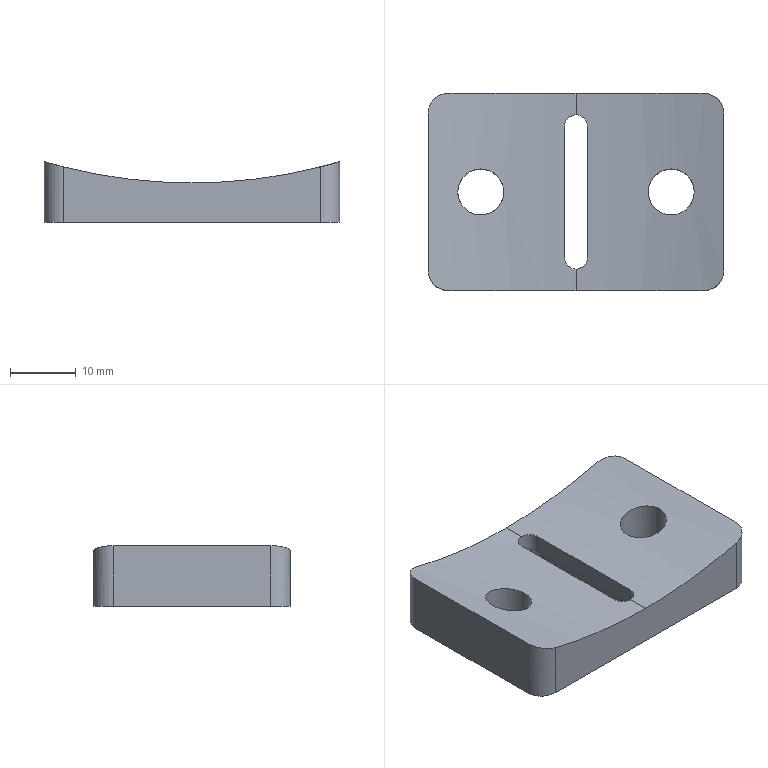Part | SolidWorks | features ICE 2, Extrusion 1, Fillet 1, HoleWzd 1 | 1 solid | 24 faces | box 45 x 30 x 9.229 mm | volume 8201 mm3 | cylinder 14 | plane 10 | commonest cylinder face diameters 6 x6 7 x4 3.5 x2 160 x2
STEP:
#1=CARTESIAN_POINT('',(18.,15.,-77.949));
#2=VERTEX_POINT('',#1);
#3=CARTESIAN_POINT('',(11.,15.,-79.24));
#4=VERTEX_POINT('',#3);
#5=CARTESIAN_POINT('',(18.,15.,-77.949));
#6=CARTESIAN_POINT('',(18.,14.77,-77.949));
#7=CARTESIAN_POINT('',(17.977,14.541,-77.954));
#8=CARTESIAN_POINT('',(17.887,14.086,-77.975));
#9=CARTESIAN_POINT('',(17.818,13.864,-77.99));
#10=CARTESIAN_POINT('',(17.642,13.441,-78.031));
#11=CARTESIAN_POINT('',(17.532,13.237,-78.055));
#12=CARTESIAN_POINT('',(17.275,12.855,-78.113));
#13=CARTESIAN_POINT('',(17.13,12.679,-78.145));
#14=CARTESIAN_POINT('',(16.807,12.358,-78.215));
#15=CARTESIAN_POINT('',(16.627,12.211,-78.253));
#16=CARTESIAN_POINT('',(16.249,11.96,-78.333));
#17=CARTESIAN_POINT('',(16.049,11.853,-78.374));
#18=CARTESIAN_POINT('',(15.628,11.679,-78.459));
#19=CARTESIAN_POINT('',(15.409,11.612,-78.502));
#20=CARTESIAN_POINT('',(14.966,11.524,-78.588));
#21=CARTESIAN_POINT('',(14.74,11.501,-78.631));
#22=CARTESIAN_POINT('',(14.282,11.499,-78.715));
#23=CARTESIAN_POINT('',(14.056,11.521,-78.756));
#24=CARTESIAN_POINT('',(13.611,11.607,-78.834));
#25=CARTESIAN_POINT('',(13.39,11.673,-78.872));
#26=CARTESIAN_POINT('',(12.967,11.845,-78.942));
#27=CARTESIAN_POINT('',(12.765,11.952,-78.975));
#28=CARTESIAN_POINT('',(12.384,12.203,-79.036));
#29=CARTESIAN_POINT('',(12.203,12.35,-79.064));
#30=CARTESIAN_POINT('',(11.877,12.672,-79.114));
#31=CARTESIAN_POINT('',(11.73,12.848,-79.135));
#32=CARTESIAN_POINT('',(11.472,13.23,-79.173));
#33=CARTESIAN_POINT('',(11.361,13.435,-79.189));
#34=CARTESIAN_POINT('',(11.095,14.07,-79.227));
#35=CARTESIAN_POINT('',(11.,14.534,-79.24));
#36=CARTESIAN_POINT('',(11.,15.,-79.24));
#37=B_SPLINE_CURVE_WITH_KNOTS('',3,(#5,#6,#7,#8,#9,#10,#11,#12,#13,#14,#15,#16,#17,#18,#19,#20,#21,#22,#23,#24,#25,#26,#27,#28,#29,#30,#31,#32,#33,#34,#35,#36),.UNSPECIFIED.,.F.,.F.,(4,2,2,2,2,2,2,2,2,2,2,2,2,2,2,4),(0.01104,0.01173,0.01242,0.01311,0.0138,0.01449,0.01518,0.01587,0.01656,0.01725,0.01793,0.01862,0.01931,0.02,0.02069,0.02207),.UNSPECIFIED.);
#38=EDGE_CURVE('',#2,#4,#37,.T.);
#39=ORIENTED_EDGE('',*,*,#38,.F.);
#40=CARTESIAN_POINT('',(18.,15.,-86.));
#41=VERTEX_POINT('',#40);
#42=CARTESIAN_POINT('',(18.,15.,-86.));
#43=DIRECTION('',(0.,0.,-1.));
#44=VECTOR('',#43,1000.);
#45=LINE('',#42,#44);
#46=EDGE_CURVE('',#2,#41,#45,.T.);
#47=ORIENTED_EDGE('',*,*,#46,.T.);
#48=CARTESIAN_POINT('',(11.,15.,-86.));
#49=VERTEX_POINT('',#48);
#50=CARTESIAN_POINT('',(14.5,15.,-86.));
#51=DIRECTION('',(0.,0.,-1.));
#52=DIRECTION('',(-1.,0.,0.));
#53=AXIS2_PLACEMENT_3D('',#50,#51,#52);
#54=CIRCLE('',#53,3.5);
#55=EDGE_CURVE('',#41,#49,#54,.T.);
#56=ORIENTED_EDGE('',*,*,#55,.T.);
#57=CARTESIAN_POINT('',(11.,15.,-86.));
#58=DIRECTION('',(0.,0.,-1.));
#59=VECTOR('',#58,1000.);
#60=LINE('',#57,#59);
#61=EDGE_CURVE('',#4,#49,#60,.T.);
#62=ORIENTED_EDGE('',*,*,#61,.F.);
#63=EDGE_LOOP('',(#39,#47,#56,#62));
#64=FACE_OUTER_BOUND('',#63,.T.);
#65=CARTESIAN_POINT('',(14.5,15.,-86.));
#66=DIRECTION('',(0.,0.,-1.));
#67=DIRECTION('',(-1.,0.,0.));
#68=AXIS2_PLACEMENT_3D('',#65,#66,#67);
#69=CYLINDRICAL_SURFACE('',#68,3.5);
#70=ADVANCED_FACE('',(#64),#69,.F.);
#71=CARTESIAN_POINT('',(-11.,15.,-79.24));
#72=VERTEX_POINT('',#71);
#73=CARTESIAN_POINT('',(-18.,15.,-77.949));
#74=VERTEX_POINT('',#73);
#75=CARTESIAN_POINT('',(-11.,15.,-79.24));
#76=CARTESIAN_POINT('',(-11.,14.77,-79.24));
#77=CARTESIAN_POINT('',(-11.023,14.541,-79.237));
#78=CARTESIAN_POINT('',(-11.114,14.086,-79.224));
#79=CARTESIAN_POINT('',(-11.182,13.863,-79.215));
#80=CARTESIAN_POINT('',(-11.359,13.439,-79.19));
#81=CARTESIAN_POINT('',(-11.469,13.235,-79.174));
#82=CARTESIAN_POINT('',(-11.728,12.851,-79.136));
#83=CARTESIAN_POINT('',(-11.874,12.675,-79.114));
#84=CARTESIAN_POINT('',(-12.199,12.353,-79.065));
#85=CARTESIAN_POINT('',(-12.38,12.205,-79.036));
#86=CARTESIAN_POINT('',(-12.762,11.953,-78.976));
#87=CARTESIAN_POINT('',(-12.963,11.847,-78.943));
#88=CARTESIAN_POINT('',(-13.387,11.674,-78.872));
#89=CARTESIAN_POINT('',(-13.608,11.608,-78.834));
#90=CARTESIAN_POINT('',(-14.053,11.521,-78.756));
#91=CARTESIAN_POINT('',(-14.279,11.499,-78.716));
#92=CARTESIAN_POINT('',(-14.737,11.501,-78.631));
#93=CARTESIAN_POINT('',(-14.963,11.523,-78.589));
#94=CARTESIAN_POINT('',(-15.406,11.612,-78.503));
#95=CARTESIAN_POINT('',(-15.626,11.678,-78.459));
#96=CARTESIAN_POINT('',(-16.046,11.852,-78.375));
#97=CARTESIAN_POINT('',(-16.246,11.958,-78.333));
#98=CARTESIAN_POINT('',(-16.624,12.209,-78.254));
#99=CARTESIAN_POINT('',(-16.804,12.356,-78.215));
#100=CARTESIAN_POINT('',(-17.127,12.676,-78.145));
#101=CARTESIAN_POINT('',(-17.272,12.851,-78.113));
#102=CARTESIAN_POINT('',(-17.53,13.232,-78.056));
#103=CARTESIAN_POINT('',(-17.64,13.437,-78.031));
#104=CARTESIAN_POINT('',(-17.905,14.07,-77.971));
#105=CARTESIAN_POINT('',(-18.,14.533,-77.949));
#106=CARTESIAN_POINT('',(-18.,15.,-77.949));
#107=B_SPLINE_CURVE_WITH_KNOTS('',3,(#75,#76,#77,#78,#79,#80,#81,#82,#83,#84,#85,#86,#87,#88,#89,#90,#91,#92,#93,#94,#95,#96,#97,#98,#99,#100,#101,#102,#103,#104,#105,#106),.UNSPECIFIED.,.F.,.F.,(4,2,2,2,2,2,2,2,2,2,2,2,2,2,2,4),(0.01104,0.01173,0.01242,0.01311,0.0138,0.01449,0.01518,0.01587,0.01656,0.01725,0.01794,0.01862,0.01931,0.02,0.02069,0.02207),.UNSPECIFIED.);
#108=EDGE_CURVE('',#72,#74,#107,.T.);
#109=ORIENTED_EDGE('',*,*,#108,.F.);
#110=CARTESIAN_POINT('',(-11.,15.,-86.));
#111=VERTEX_POINT('',#110);
#112=CARTESIAN_POINT('',(-11.,15.,-86.));
#113=DIRECTION('',(0.,0.,-1.));
#114=VECTOR('',#113,1000.);
#115=LINE('',#112,#114);
#116=EDGE_CURVE('',#72,#111,#115,.T.);
#117=ORIENTED_EDGE('',*,*,#116,.T.);
#118=CARTESIAN_POINT('',(-18.,15.,-86.));
#119=VERTEX_POINT('',#118);
#120=CARTESIAN_POINT('',(-14.5,15.,-86.));
#121=DIRECTION('',(0.,0.,-1.));
#122=DIRECTION('',(-1.,0.,0.));
#123=AXIS2_PLACEMENT_3D('',#120,#121,#122);
#124=CIRCLE('',#123,3.5);
#125=EDGE_CURVE('',#111,#119,#124,.T.);
#126=ORIENTED_EDGE('',*,*,#125,.T.);
#127=CARTESIAN_POINT('',(-18.,15.,-86.));
#128=DIRECTION('',(0.,0.,-1.));
#129=VECTOR('',#128,1000.);
#130=LINE('',#127,#129);
#131=EDGE_CURVE('',#74,#119,#130,.T.);
#132=ORIENTED_EDGE('',*,*,#131,.F.);
#133=EDGE_LOOP('',(#109,#117,#126,#132));
#134=FACE_OUTER_BOUND('',#133,.T.);
#135=CARTESIAN_POINT('',(-14.5,15.,-86.));
#136=DIRECTION('',(0.,0.,-1.));
#137=DIRECTION('',(-1.,0.,0.));
#138=AXIS2_PLACEMENT_3D('',#135,#136,#137);
#139=CYLINDRICAL_SURFACE('',#138,3.5);
#140=ADVANCED_FACE('',(#134),#139,.F.);
#141=CARTESIAN_POINT('',(11.,15.,-79.24));
#142=CARTESIAN_POINT('',(11.,15.233,-79.24));
#143=CARTESIAN_POINT('',(11.023,15.463,-79.237));
#144=CARTESIAN_POINT('',(11.114,15.914,-79.224));
#145=CARTESIAN_POINT('',(11.182,16.138,-79.215));
#146=CARTESIAN_POINT('',(11.36,16.564,-79.189));
#147=CARTESIAN_POINT('',(11.469,16.766,-79.174));
#148=CARTESIAN_POINT('',(11.727,17.147,-79.136));
#149=CARTESIAN_POINT('',(11.876,17.327,-79.114));
#150=CARTESIAN_POINT('',(12.201,17.649,-79.064));
#151=CARTESIAN_POINT('',(12.379,17.794,-79.037));
#152=CARTESIAN_POINT('',(12.764,18.048,-78.975));
#153=CARTESIAN_POINT('',(12.967,18.155,-78.942));
#154=CARTESIAN_POINT('',(13.388,18.326,-78.872));
#155=CARTESIAN_POINT('',(13.609,18.392,-78.834));
#156=CARTESIAN_POINT('',(14.057,18.479,-78.756));
#157=CARTESIAN_POINT('',(14.283,18.501,-78.715));
#158=CARTESIAN_POINT('',(14.736,18.499,-78.631));
#159=CARTESIAN_POINT('',(14.966,18.476,-78.588));
#160=CARTESIAN_POINT('',(15.41,18.387,-78.502));
#161=CARTESIAN_POINT('',(15.626,18.322,-78.459));
#162=CARTESIAN_POINT('',(16.047,18.148,-78.374));
#163=CARTESIAN_POINT('',(16.25,18.04,-78.332));
#164=CARTESIAN_POINT('',(16.627,17.789,-78.253));
#165=CARTESIAN_POINT('',(16.803,17.645,-78.216));
#166=CARTESIAN_POINT('',(17.13,17.321,-78.145));
#167=CARTESIAN_POINT('',(17.276,17.144,-78.113));
#168=CARTESIAN_POINT('',(17.53,16.766,-78.056));
#169=CARTESIAN_POINT('',(17.641,16.562,-78.031));
#170=CARTESIAN_POINT('',(17.819,16.135,-77.99));
#171=CARTESIAN_POINT('',(17.886,15.916,-77.975));
#172=CARTESIAN_POINT('',(17.977,15.465,-77.954));
#173=CARTESIAN_POINT('',(18.,15.23,-77.949));
#174=CARTESIAN_POINT('',(18.,15.,-77.949));
#175=B_SPLINE_CURVE_WITH_KNOTS('',3,(#141,#142,#143,#144,#145,#146,#147,#148,#149,#150,#151,#152,#153,#154,#155,#156,#157,#158,#159,#160,#161,#162,#163,#164,#165,#166,#167,#168,#169,#170,#171,#172,#173,#174),.UNSPECIFIED.,.F.,.F.,(4,2,2,2,2,2,2,2,2,2,2,2,2,2,2,2,4),(0.,0.0006899,0.00138,0.00207,0.00276,0.003449,0.004139,0.004829,0.005519,0.006209,0.006899,0.007589,0.008279,0.008969,0.009658,0.01035,0.01104),.UNSPECIFIED.);
#176=EDGE_CURVE('',#4,#2,#175,.T.);
#177=ORIENTED_EDGE('',*,*,#176,.T.);
#178=ORIENTED_EDGE('',*,*,#38,.T.);
#179=EDGE_LOOP('',(#177,#178));
#180=FACE_BOUND('',#179,.T.);
#181=CARTESIAN_POINT('',(0.,30.,-80.));
#182=VERTEX_POINT('',#181);
#183=CARTESIAN_POINT('',(19.5,30.,-77.587));
#184=VERTEX_POINT('',#183);
#185=CARTESIAN_POINT('',(0.,30.,0.));
#186=DIRECTION('',(0.,-1.,0.));
#187=DIRECTION('',(0.,0.,1.));
#188=AXIS2_PLACEMENT_3D('',#185,#186,#187);
#189=CIRCLE('',#188,80.);
#190=EDGE_CURVE('',#182,#184,#189,.T.);
#191=ORIENTED_EDGE('',*,*,#190,.F.);
#192=CARTESIAN_POINT('',(0.,26.75,-80.));
#193=VERTEX_POINT('',#192);
#194=CARTESIAN_POINT('',(0.,30.,-80.));
#195=DIRECTION('',(0.,-1.,0.));
#196=VECTOR('',#195,1000.);
#197=LINE('',#194,#196);
#198=EDGE_CURVE('',#182,#193,#197,.T.);
#199=ORIENTED_EDGE('',*,*,#198,.T.);
#200=CARTESIAN_POINT('',(1.75,25.,-79.981));
#201=VERTEX_POINT('',#200);
#202=CARTESIAN_POINT('',(0.,26.75,-80.));
#203=CARTESIAN_POINT('',(0.1141,26.75,-80.));
#204=CARTESIAN_POINT('',(0.2299,26.739,-80.));
#205=CARTESIAN_POINT('',(0.4542,26.694,-79.999));
#206=CARTESIAN_POINT('',(0.5633,26.661,-79.998));
#207=CARTESIAN_POINT('',(0.775,26.573,-79.996));
#208=CARTESIAN_POINT('',(0.8774,26.518,-79.995));
#209=CARTESIAN_POINT('',(1.067,26.392,-79.993));
#210=CARTESIAN_POINT('',(1.155,26.32,-79.992));
#211=CARTESIAN_POINT('',(1.319,26.156,-79.989));
#212=CARTESIAN_POINT('',(1.391,26.068,-79.988));
#213=CARTESIAN_POINT('',(1.518,25.878,-79.986));
#214=CARTESIAN_POINT('',(1.573,25.776,-79.985));
#215=CARTESIAN_POINT('',(1.704,25.458,-79.982));
#216=CARTESIAN_POINT('',(1.75,25.231,-79.981));
#217=CARTESIAN_POINT('',(1.75,25.,-79.981));
#218=B_SPLINE_CURVE_WITH_KNOTS('',3,(#202,#203,#204,#205,#206,#207,#208,#209,#210,#211,#212,#213,#214,#215,#216,#217),.UNSPECIFIED.,.F.,.F.,(4,2,2,2,2,2,2,4),(0.002736,0.003078,0.00342,0.003762,0.004103,0.004445,0.004787,0.00547),.UNSPECIFIED.);
#219=EDGE_CURVE('',#193,#201,#218,.T.);
#220=ORIENTED_EDGE('',*,*,#219,.T.);
#221=CARTESIAN_POINT('',(1.75,5.,-79.981));
#222=VERTEX_POINT('',#221);
#223=CARTESIAN_POINT('',(1.75,30.,-79.981));
#224=DIRECTION('',(0.,-1.,0.));
#225=VECTOR('',#224,1000.);
#226=LINE('',#223,#225);
#227=EDGE_CURVE('',#201,#222,#226,.T.);
#228=ORIENTED_EDGE('',*,*,#227,.T.);
#229=CARTESIAN_POINT('',(0.,3.25,-80.));
#230=VERTEX_POINT('',#229);
#231=CARTESIAN_POINT('',(1.75,5.,-79.981));
#232=CARTESIAN_POINT('',(1.75,4.884,-79.981));
#233=CARTESIAN_POINT('',(1.739,4.771,-79.981));
#234=CARTESIAN_POINT('',(1.694,4.547,-79.982));
#235=CARTESIAN_POINT('',(1.66,4.436,-79.983));
#236=CARTESIAN_POINT('',(1.573,4.224,-79.985));
#237=CARTESIAN_POINT('',(1.519,4.123,-79.986));
#238=CARTESIAN_POINT('',(1.392,3.933,-79.988));
#239=CARTESIAN_POINT('',(1.318,3.843,-79.989));
#240=CARTESIAN_POINT('',(1.075,3.601,-79.993));
#241=CARTESIAN_POINT('',(0.8801,3.47,-79.995));
#242=CARTESIAN_POINT('',(0.4587,3.296,-79.999));
#243=CARTESIAN_POINT('',(0.2283,3.25,-80.));
#244=CARTESIAN_POINT('',(0.,3.25,-80.));
#245=B_SPLINE_CURVE_WITH_KNOTS('',3,(#231,#232,#233,#234,#235,#236,#237,#238,#239,#240,#241,#242,#243,#244),.UNSPECIFIED.,.F.,.F.,(4,2,2,2,2,2,4),(0.,0.000342,0.0006841,0.001026,0.001368,0.002052,0.002736),.UNSPECIFIED.);
#246=EDGE_CURVE('',#222,#230,#245,.T.);
#247=ORIENTED_EDGE('',*,*,#246,.T.);
#248=CARTESIAN_POINT('',(0.,0.,-80.));
#249=VERTEX_POINT('',#248);
#250=CARTESIAN_POINT('',(0.,30.,-80.));
#251=DIRECTION('',(0.,-1.,0.));
#252=VECTOR('',#251,1000.);
#253=LINE('',#250,#252);
#254=EDGE_CURVE('',#230,#249,#253,.T.);
#255=ORIENTED_EDGE('',*,*,#254,.T.);
#256=CARTESIAN_POINT('',(19.5,0.,-77.587));
#257=VERTEX_POINT('',#256);
#258=CARTESIAN_POINT('',(0.,0.,0.));
#259=DIRECTION('',(0.,-1.,0.));
#260=DIRECTION('',(0.,0.,1.));
#261=AXIS2_PLACEMENT_3D('',#258,#259,#260);
#262=CIRCLE('',#261,80.);
#263=EDGE_CURVE('',#249,#257,#262,.T.);
#264=ORIENTED_EDGE('',*,*,#263,.T.);
#265=CARTESIAN_POINT('',(22.5,3.,-76.771));
#266=VERTEX_POINT('',#265);
#267=CARTESIAN_POINT('',(19.5,0.,-77.587));
#268=CARTESIAN_POINT('',(19.696,0.,-77.538));
#269=CARTESIAN_POINT('',(19.888,0.01893,-77.489));
#270=CARTESIAN_POINT('',(20.266,0.09302,-77.391));
#271=CARTESIAN_POINT('',(20.453,0.1489,-77.341));
#272=CARTESIAN_POINT('',(20.814,0.296,-77.245));
#273=CARTESIAN_POINT('',(20.985,0.386,-77.199));
#274=CARTESIAN_POINT('',(21.309,0.5991,-77.11));
#275=CARTESIAN_POINT('',(21.464,0.7237,-77.067));
#276=CARTESIAN_POINT('',(21.743,0.998,-76.989));
#277=CARTESIAN_POINT('',(21.868,1.148,-76.953));
#278=CARTESIAN_POINT('',(22.09,1.474,-76.89));
#279=CARTESIAN_POINT('',(22.187,1.65,-76.862));
#280=CARTESIAN_POINT('',(22.417,2.197,-76.795));
#281=CARTESIAN_POINT('',(22.5,2.596,-76.771));
#282=CARTESIAN_POINT('',(22.5,3.,-76.771));
#283=B_SPLINE_CURVE_WITH_KNOTS('',3,(#267,#268,#269,#270,#271,#272,#273,#274,#275,#276,#277,#278,#279,#280,#281,#282),.UNSPECIFIED.,.F.,.F.,(4,2,2,2,2,2,2,4),(0.,0.0005963,0.001193,0.001789,0.002385,0.002981,0.003578,0.00477),.UNSPECIFIED.);
#284=EDGE_CURVE('',#257,#266,#283,.T.);
#285=ORIENTED_EDGE('',*,*,#284,.T.);
#286=CARTESIAN_POINT('',(22.5,27.,-76.771));
#287=VERTEX_POINT('',#286);
#288=CARTESIAN_POINT('',(22.5,30.,-76.771));
#289=DIRECTION('',(0.,-1.,0.));
#290=VECTOR('',#289,1000.);
#291=LINE('',#288,#290);
#292=EDGE_CURVE('',#287,#266,#291,.T.);
#293=ORIENTED_EDGE('',*,*,#292,.F.);
#294=CARTESIAN_POINT('',(22.5,27.,-76.771));
#295=CARTESIAN_POINT('',(22.5,27.202,-76.771));
#296=CARTESIAN_POINT('',(22.48,27.4,-76.777));
#297=CARTESIAN_POINT('',(22.401,27.789,-76.8));
#298=CARTESIAN_POINT('',(22.342,27.982,-76.817));
#299=CARTESIAN_POINT('',(22.187,28.348,-76.862));
#300=CARTESIAN_POINT('',(22.093,28.521,-76.889));
#301=CARTESIAN_POINT('',(21.871,28.848,-76.952));
#302=CARTESIAN_POINT('',(21.744,29.001,-76.989));
#303=CARTESIAN_POINT('',(21.327,29.412,-77.105));
#304=CARTESIAN_POINT('',(20.993,29.63,-77.197));
#305=CARTESIAN_POINT('',(20.457,29.85,-77.34));
#306=CARTESIAN_POINT('',(20.269,29.906,-77.39));
#307=CARTESIAN_POINT('',(19.888,29.981,-77.489));
#308=CARTESIAN_POINT('',(19.695,30.,-77.538));
#309=CARTESIAN_POINT('',(19.5,30.,-77.587));
#310=B_SPLINE_CURVE_WITH_KNOTS('',3,(#294,#295,#296,#297,#298,#299,#300,#301,#302,#303,#304,#305,#306,#307,#308,#309),.UNSPECIFIED.,.F.,.F.,(4,2,2,2,2,2,2,4),(0.,0.0005963,0.001193,0.001789,0.002385,0.003578,0.004174,0.00477),.UNSPECIFIED.);
#311=EDGE_CURVE('',#287,#184,#310,.T.);
#312=ORIENTED_EDGE('',*,*,#311,.T.);
#313=EDGE_LOOP('',(#191,#199,#220,#228,#247,#255,#264,#285,#293,#312));
#314=FACE_OUTER_BOUND('',#313,.T.);
#315=CARTESIAN_POINT('',(0.,30.,0.));
#316=DIRECTION('',(0.,-1.,0.));
#317=DIRECTION('',(0.,0.,-1.));
#318=AXIS2_PLACEMENT_3D('',#315,#316,#317);
#319=CYLINDRICAL_SURFACE('',#318,80.);
#320=ADVANCED_FACE('',(#180,#314),#319,.F.);
#321=CARTESIAN_POINT('',(1.75,25.,-82.7));
#322=VERTEX_POINT('',#321);
#323=CARTESIAN_POINT('',(-1.75,25.,-82.7));
#324=VERTEX_POINT('',#323);
#325=CARTESIAN_POINT('',(0.,25.,-82.7));
#326=DIRECTION('',(0.,0.,1.));
#327=DIRECTION('',(-1.,0.,0.));
#328=AXIS2_PLACEMENT_3D('',#325,#326,#327);
#329=CIRCLE('',#328,1.75);
#330=EDGE_CURVE('',#322,#324,#329,.T.);
#331=ORIENTED_EDGE('',*,*,#330,.F.);
#332=CARTESIAN_POINT('',(1.75,25.,-76.771));
#333=DIRECTION('',(0.,0.,-1.));
#334=VECTOR('',#333,1000.);
#335=LINE('',#332,#334);
#336=EDGE_CURVE('',#201,#322,#335,.T.);
#337=ORIENTED_EDGE('',*,*,#336,.F.);
#338=ORIENTED_EDGE('',*,*,#219,.F.);
#339=CARTESIAN_POINT('',(-1.75,25.,-79.981));
#340=VERTEX_POINT('',#339);
#341=CARTESIAN_POINT('',(-1.75,25.,-79.981));
#342=CARTESIAN_POINT('',(-1.75,25.116,-79.981));
#343=CARTESIAN_POINT('',(-1.739,25.229,-79.981));
#344=CARTESIAN_POINT('',(-1.694,25.453,-79.982));
#345=CARTESIAN_POINT('',(-1.66,25.564,-79.983));
#346=CARTESIAN_POINT('',(-1.573,25.776,-79.985));
#347=CARTESIAN_POINT('',(-1.519,25.877,-79.986));
#348=CARTESIAN_POINT('',(-1.392,26.067,-79.988));
#349=CARTESIAN_POINT('',(-1.318,26.157,-79.989));
#350=CARTESIAN_POINT('',(-1.075,26.399,-79.993));
#351=CARTESIAN_POINT('',(-0.8801,26.53,-79.995));
#352=CARTESIAN_POINT('',(-0.4587,26.704,-79.999));
#353=CARTESIAN_POINT('',(-0.2283,26.75,-80.));
#354=CARTESIAN_POINT('',(0.,26.75,-80.));
#355=B_SPLINE_CURVE_WITH_KNOTS('',3,(#341,#342,#343,#344,#345,#346,#347,#348,#349,#350,#351,#352,#353,#354),.UNSPECIFIED.,.F.,.F.,(4,2,2,2,2,2,4),(0.,0.000342,0.0006841,0.001026,0.001368,0.002052,0.002736),.UNSPECIFIED.);
#356=EDGE_CURVE('',#340,#193,#355,.T.);
#357=ORIENTED_EDGE('',*,*,#356,.F.);
#358=CARTESIAN_POINT('',(-1.75,25.,-76.771));
#359=DIRECTION('',(0.,0.,-1.));
#360=VECTOR('',#359,1000.);
#361=LINE('',#358,#360);
#362=EDGE_CURVE('',#340,#324,#361,.T.);
#363=ORIENTED_EDGE('',*,*,#362,.T.);
#364=EDGE_LOOP('',(#331,#337,#338,#357,#363));
#365=FACE_OUTER_BOUND('',#364,.T.);
#366=CARTESIAN_POINT('',(0.,25.,-76.771));
#367=DIRECTION('',(0.,0.,-1.));
#368=DIRECTION('',(-1.,0.,0.));
#369=AXIS2_PLACEMENT_3D('',#366,#367,#368);
#370=CYLINDRICAL_SURFACE('',#369,1.75);
#371=ADVANCED_FACE('',(#365),#370,.F.);
#372=CARTESIAN_POINT('',(-1.75,5.,-82.7));
#373=VERTEX_POINT('',#372);
#374=CARTESIAN_POINT('',(-1.75,25.,-82.7));
#375=DIRECTION('',(0.,-1.,0.));
#376=VECTOR('',#375,1000.);
#377=LINE('',#374,#376);
#378=EDGE_CURVE('',#324,#373,#377,.T.);
#379=ORIENTED_EDGE('',*,*,#378,.F.);
#380=ORIENTED_EDGE('',*,*,#362,.F.);
#381=CARTESIAN_POINT('',(-1.75,5.,-79.981));
#382=VERTEX_POINT('',#381);
#383=CARTESIAN_POINT('',(-1.75,30.,-79.981));
#384=DIRECTION('',(0.,1.,0.));
#385=VECTOR('',#384,1000.);
#386=LINE('',#383,#385);
#387=EDGE_CURVE('',#382,#340,#386,.T.);
#388=ORIENTED_EDGE('',*,*,#387,.F.);
#389=CARTESIAN_POINT('',(-1.75,5.,-76.771));
#390=DIRECTION('',(0.,0.,-1.));
#391=VECTOR('',#390,1000.);
#392=LINE('',#389,#391);
#393=EDGE_CURVE('',#382,#373,#392,.T.);
#394=ORIENTED_EDGE('',*,*,#393,.T.);
#395=EDGE_LOOP('',(#379,#380,#388,#394));
#396=FACE_OUTER_BOUND('',#395,.T.);
#397=CARTESIAN_POINT('',(-1.75,25.,-76.771));
#398=DIRECTION('',(-1.,0.,0.));
#399=DIRECTION('',(0.,0.,1.));
#400=AXIS2_PLACEMENT_3D('',#397,#398,#399);
#401=PLANE('',#400);
#402=ADVANCED_FACE('',(#396),#401,.F.);
#403=CARTESIAN_POINT('',(1.75,5.,-82.7));
#404=VERTEX_POINT('',#403);
#405=CARTESIAN_POINT('',(0.,5.,-82.7));
#406=DIRECTION('',(0.,0.,1.));
#407=DIRECTION('',(-1.,0.,0.));
#408=AXIS2_PLACEMENT_3D('',#405,#406,#407);
#409=CIRCLE('',#408,1.75);
#410=EDGE_CURVE('',#373,#404,#409,.T.);
#411=ORIENTED_EDGE('',*,*,#410,.F.);
#412=ORIENTED_EDGE('',*,*,#393,.F.);
#413=CARTESIAN_POINT('',(0.,3.25,-80.));
#414=CARTESIAN_POINT('',(-0.1141,3.25,-80.));
#415=CARTESIAN_POINT('',(-0.2299,3.261,-80.));
#416=CARTESIAN_POINT('',(-0.4542,3.306,-79.999));
#417=CARTESIAN_POINT('',(-0.5633,3.339,-79.998));
#418=CARTESIAN_POINT('',(-0.775,3.427,-79.996));
#419=CARTESIAN_POINT('',(-0.8774,3.482,-79.995));
#420=CARTESIAN_POINT('',(-1.067,3.608,-79.993));
#421=CARTESIAN_POINT('',(-1.155,3.68,-79.992));
#422=CARTESIAN_POINT('',(-1.319,3.844,-79.989));
#423=CARTESIAN_POINT('',(-1.391,3.932,-79.988));
#424=CARTESIAN_POINT('',(-1.518,4.122,-79.986));
#425=CARTESIAN_POINT('',(-1.573,4.224,-79.985));
#426=CARTESIAN_POINT('',(-1.704,4.542,-79.982));
#427=CARTESIAN_POINT('',(-1.75,4.769,-79.981));
#428=CARTESIAN_POINT('',(-1.75,5.,-79.981));
#429=B_SPLINE_CURVE_WITH_KNOTS('',3,(#413,#414,#415,#416,#417,#418,#419,#420,#421,#422,#423,#424,#425,#426,#427,#428),.UNSPECIFIED.,.F.,.F.,(4,2,2,2,2,2,2,4),(0.002736,0.003078,0.00342,0.003762,0.004103,0.004445,0.004787,0.00547),.UNSPECIFIED.);
#430=EDGE_CURVE('',#230,#382,#429,.T.);
#431=ORIENTED_EDGE('',*,*,#430,.F.);
#432=ORIENTED_EDGE('',*,*,#246,.F.);
#433=CARTESIAN_POINT('',(1.75,5.,-76.771));
#434=DIRECTION('',(0.,0.,-1.));
#435=VECTOR('',#434,1000.);
#436=LINE('',#433,#435);
#437=EDGE_CURVE('',#222,#404,#436,.T.);
#438=ORIENTED_EDGE('',*,*,#437,.T.);
#439=EDGE_LOOP('',(#411,#412,#431,#432,#438));
#440=FACE_OUTER_BOUND('',#439,.T.);
#441=CARTESIAN_POINT('',(0.,5.,-76.771));
#442=DIRECTION('',(0.,0.,-1.));
#443=DIRECTION('',(-1.,0.,0.));
#444=AXIS2_PLACEMENT_3D('',#441,#442,#443);
#445=CYLINDRICAL_SURFACE('',#444,1.75);
#446=ADVANCED_FACE('',(#440),#445,.F.);
#447=CARTESIAN_POINT('',(1.75,25.,-82.7));
#448=DIRECTION('',(0.,1.,0.));
#449=VECTOR('',#448,1000.);
#450=LINE('',#447,#449);
#451=EDGE_CURVE('',#404,#322,#450,.T.);
#452=ORIENTED_EDGE('',*,*,#451,.F.);
#453=ORIENTED_EDGE('',*,*,#437,.F.);
#454=ORIENTED_EDGE('',*,*,#227,.F.);
#455=ORIENTED_EDGE('',*,*,#336,.T.);
#456=EDGE_LOOP('',(#452,#453,#454,#455));
#457=FACE_OUTER_BOUND('',#456,.T.);
#458=CARTESIAN_POINT('',(1.75,25.,-76.771));
#459=DIRECTION('',(1.,0.,0.));
#460=DIRECTION('',(0.,0.,-1.));
#461=AXIS2_PLACEMENT_3D('',#458,#459,#460);
#462=PLANE('',#461);
#463=ADVANCED_FACE('',(#457),#462,.F.);
#464=CARTESIAN_POINT('',(3.,25.,-86.));
#465=VERTEX_POINT('',#464);
#466=CARTESIAN_POINT('',(3.,5.,-86.));
#467=VERTEX_POINT('',#466);
#468=CARTESIAN_POINT('',(3.,25.,-86.));
#469=DIRECTION('',(0.,-1.,0.));
#470=VECTOR('',#469,1000.);
#471=LINE('',#468,#470);
#472=EDGE_CURVE('',#465,#467,#471,.T.);
#473=ORIENTED_EDGE('',*,*,#472,.F.);
#474=CARTESIAN_POINT('',(-3.,25.,-86.));
#475=VERTEX_POINT('',#474);
#476=CARTESIAN_POINT('',(0.,25.,-86.));
#477=DIRECTION('',(0.,0.,-1.));
#478=DIRECTION('',(-1.,0.,0.));
#479=AXIS2_PLACEMENT_3D('',#476,#477,#478);
#480=CIRCLE('',#479,3.);
#481=EDGE_CURVE('',#475,#465,#480,.T.);
#482=ORIENTED_EDGE('',*,*,#481,.F.);
#483=CARTESIAN_POINT('',(-3.,5.,-86.));
#484=VERTEX_POINT('',#483);
#485=CARTESIAN_POINT('',(-3.,25.,-86.));
#486=DIRECTION('',(0.,1.,0.));
#487=VECTOR('',#486,1000.);
#488=LINE('',#485,#487);
#489=EDGE_CURVE('',#484,#475,#488,.T.);
#490=ORIENTED_EDGE('',*,*,#489,.F.);
#491=CARTESIAN_POINT('',(0.,5.,-86.));
#492=DIRECTION('',(0.,0.,-1.));
#493=DIRECTION('',(-1.,0.,0.));
#494=AXIS2_PLACEMENT_3D('',#491,#492,#493);
#495=CIRCLE('',#494,3.);
#496=EDGE_CURVE('',#467,#484,#495,.T.);
#497=ORIENTED_EDGE('',*,*,#496,.F.);
#498=EDGE_LOOP('',(#473,#482,#490,#497));
#499=FACE_BOUND('',#498,.T.);
#500=CARTESIAN_POINT('',(14.5,15.,-86.));
#501=DIRECTION('',(0.,0.,-1.));
#502=DIRECTION('',(-1.,0.,0.));
#503=AXIS2_PLACEMENT_3D('',#500,#501,#502);
#504=CIRCLE('',#503,3.5);
#505=EDGE_CURVE('',#49,#41,#504,.T.);
#506=ORIENTED_EDGE('',*,*,#505,.F.);
#507=ORIENTED_EDGE('',*,*,#55,.F.);
#508=EDGE_LOOP('',(#506,#507));
#509=FACE_BOUND('',#508,.T.);
#510=CARTESIAN_POINT('',(-14.5,15.,-86.));
#511=DIRECTION('',(0.,0.,-1.));
#512=DIRECTION('',(-1.,0.,0.));
#513=AXIS2_PLACEMENT_3D('',#510,#511,#512);
#514=CIRCLE('',#513,3.5);
#515=EDGE_CURVE('',#119,#111,#514,.T.);
#516=ORIENTED_EDGE('',*,*,#515,.F.);
#517=ORIENTED_EDGE('',*,*,#125,.F.);
#518=EDGE_LOOP('',(#516,#517));
#519=FACE_BOUND('',#518,.T.);
#520=CARTESIAN_POINT('',(-22.5,27.,-86.));
#521=VERTEX_POINT('',#520);
#522=CARTESIAN_POINT('',(-22.5,3.,-86.));
#523=VERTEX_POINT('',#522);
#524=CARTESIAN_POINT('',(-22.5,30.,-86.));
#525=DIRECTION('',(0.,-1.,0.));
#526=VECTOR('',#525,1000.);
#527=LINE('',#524,#526);
#528=EDGE_CURVE('',#521,#523,#527,.T.);
#529=ORIENTED_EDGE('',*,*,#528,.F.);
#530=CARTESIAN_POINT('',(-19.5,30.,-86.));
#531=VERTEX_POINT('',#530);
#532=CARTESIAN_POINT('',(-19.5,27.,-86.));
#533=DIRECTION('',(0.,0.,-1.));
#534=DIRECTION('',(1.,0.,0.));
#535=AXIS2_PLACEMENT_3D('',#532,#533,#534);
#536=CIRCLE('',#535,3.);
#537=EDGE_CURVE('',#521,#531,#536,.T.);
#538=ORIENTED_EDGE('',*,*,#537,.T.);
#539=CARTESIAN_POINT('',(19.5,30.,-86.));
#540=VERTEX_POINT('',#539);
#541=CARTESIAN_POINT('',(-22.5,30.,-86.));
#542=DIRECTION('',(-1.,0.,0.));
#543=VECTOR('',#542,1000.);
#544=LINE('',#541,#543);
#545=EDGE_CURVE('',#540,#531,#544,.T.);
#546=ORIENTED_EDGE('',*,*,#545,.F.);
#547=CARTESIAN_POINT('',(22.5,27.,-86.));
#548=VERTEX_POINT('',#547);
#549=CARTESIAN_POINT('',(19.5,27.,-86.));
#550=DIRECTION('',(0.,0.,-1.));
#551=DIRECTION('',(1.,0.,0.));
#552=AXIS2_PLACEMENT_3D('',#549,#550,#551);
#553=CIRCLE('',#552,3.);
#554=EDGE_CURVE('',#540,#548,#553,.T.);
#555=ORIENTED_EDGE('',*,*,#554,.T.);
#556=CARTESIAN_POINT('',(22.5,3.,-86.));
#557=VERTEX_POINT('',#556);
#558=CARTESIAN_POINT('',(22.5,30.,-86.));
#559=DIRECTION('',(0.,-1.,0.));
#560=VECTOR('',#559,1000.);
#561=LINE('',#558,#560);
#562=EDGE_CURVE('',#548,#557,#561,.T.);
#563=ORIENTED_EDGE('',*,*,#562,.T.);
#564=CARTESIAN_POINT('',(19.5,0.,-86.));
#565=VERTEX_POINT('',#564);
#566=CARTESIAN_POINT('',(19.5,3.,-86.));
#567=DIRECTION('',(0.,0.,-1.));
#568=DIRECTION('',(1.,0.,0.));
#569=AXIS2_PLACEMENT_3D('',#566,#567,#568);
#570=CIRCLE('',#569,3.);
#571=EDGE_CURVE('',#557,#565,#570,.T.);
#572=ORIENTED_EDGE('',*,*,#571,.T.);
#573=CARTESIAN_POINT('',(-19.5,0.,-86.));
#574=VERTEX_POINT('',#573);
#575=CARTESIAN_POINT('',(-22.5,0.,-86.));
#576=DIRECTION('',(-1.,0.,0.));
#577=VECTOR('',#576,1000.);
#578=LINE('',#575,#577);
#579=EDGE_CURVE('',#565,#574,#578,.T.);
#580=ORIENTED_EDGE('',*,*,#579,.T.);
#581=CARTESIAN_POINT('',(-19.5,3.,-86.));
#582=DIRECTION('',(0.,0.,-1.));
#583=DIRECTION('',(1.,0.,0.));
#584=AXIS2_PLACEMENT_3D('',#581,#582,#583);
#585=CIRCLE('',#584,3.);
#586=EDGE_CURVE('',#574,#523,#585,.T.);
#587=ORIENTED_EDGE('',*,*,#586,.T.);
#588=EDGE_LOOP('',(#529,#538,#546,#555,#563,#572,#580,#587));
#589=FACE_OUTER_BOUND('',#588,.T.);
#590=CARTESIAN_POINT('',(-22.5,30.,-86.));
#591=DIRECTION('',(0.,0.,1.));
#592=DIRECTION('',(1.,0.,0.));
#593=AXIS2_PLACEMENT_3D('',#590,#591,#592);
#594=PLANE('',#593);
#595=ADVANCED_FACE('',(#499,#509,#519,#589),#594,.F.);
#596=CARTESIAN_POINT('',(-22.5,27.,-76.771));
#597=VERTEX_POINT('',#596);
#598=CARTESIAN_POINT('',(-22.5,3.,-76.771));
#599=VERTEX_POINT('',#598);
#600=CARTESIAN_POINT('',(-22.5,30.,-76.771));
#601=DIRECTION('',(0.,-1.,0.));
#602=VECTOR('',#601,1000.);
#603=LINE('',#600,#602);
#604=EDGE_CURVE('',#597,#599,#603,.T.);
#605=ORIENTED_EDGE('',*,*,#604,.F.);
#606=CARTESIAN_POINT('',(-22.5,27.,-86.));
#607=DIRECTION('',(0.,0.,-1.));
#608=VECTOR('',#607,1000.);
#609=LINE('',#606,#608);
#610=EDGE_CURVE('',#597,#521,#609,.T.);
#611=ORIENTED_EDGE('',*,*,#610,.T.);
#612=ORIENTED_EDGE('',*,*,#528,.T.);
#613=CARTESIAN_POINT('',(-22.5,3.,-76.771));
#614=DIRECTION('',(0.,0.,1.));
#615=VECTOR('',#614,1000.);
#616=LINE('',#613,#615);
#617=EDGE_CURVE('',#523,#599,#616,.T.);
#618=ORIENTED_EDGE('',*,*,#617,.T.);
#619=EDGE_LOOP('',(#605,#611,#612,#618));
#620=FACE_OUTER_BOUND('',#619,.T.);
#621=CARTESIAN_POINT('',(-22.5,30.,-76.771));
#622=DIRECTION('',(1.,0.,0.));
#623=DIRECTION('',(0.,0.,-1.));
#624=AXIS2_PLACEMENT_3D('',#621,#622,#623);
#625=PLANE('',#624);
#626=ADVANCED_FACE('',(#620),#625,.F.);
#627=ORIENTED_EDGE('',*,*,#198,.F.);
#628=CARTESIAN_POINT('',(-19.5,30.,-77.587));
#629=VERTEX_POINT('',#628);
#630=CARTESIAN_POINT('',(0.,30.,0.));
#631=DIRECTION('',(0.,-1.,0.));
#632=DIRECTION('',(0.,0.,1.));
#633=AXIS2_PLACEMENT_3D('',#630,#631,#632);
#634=CIRCLE('',#633,80.);
#635=EDGE_CURVE('',#629,#182,#634,.T.);
#636=ORIENTED_EDGE('',*,*,#635,.F.);
#637=CARTESIAN_POINT('',(-19.5,30.,-77.587));
#638=CARTESIAN_POINT('',(-19.696,30.,-77.538));
#639=CARTESIAN_POINT('',(-19.888,29.981,-77.489));
#640=CARTESIAN_POINT('',(-20.266,29.907,-77.391));
#641=CARTESIAN_POINT('',(-20.453,29.851,-77.341));
#642=CARTESIAN_POINT('',(-20.814,29.704,-77.245));
#643=CARTESIAN_POINT('',(-20.985,29.614,-77.199));
#644=CARTESIAN_POINT('',(-21.309,29.401,-77.11));
#645=CARTESIAN_POINT('',(-21.464,29.276,-77.067));
#646=CARTESIAN_POINT('',(-21.743,29.002,-76.989));
#647=CARTESIAN_POINT('',(-21.868,28.852,-76.953));
#648=CARTESIAN_POINT('',(-22.09,28.526,-76.89));
#649=CARTESIAN_POINT('',(-22.187,28.35,-76.862));
#650=CARTESIAN_POINT('',(-22.417,27.803,-76.795));
#651=CARTESIAN_POINT('',(-22.5,27.404,-76.771));
#652=CARTESIAN_POINT('',(-22.5,27.,-76.771));
#653=B_SPLINE_CURVE_WITH_KNOTS('',3,(#637,#638,#639,#640,#641,#642,#643,#644,#645,#646,#647,#648,#649,#650,#651,#652),.UNSPECIFIED.,.F.,.F.,(4,2,2,2,2,2,2,4),(0.,0.0005963,0.001193,0.001789,0.002385,0.002981,0.003578,0.00477),.UNSPECIFIED.);
#654=EDGE_CURVE('',#629,#597,#653,.T.);
#655=ORIENTED_EDGE('',*,*,#654,.T.);
#656=ORIENTED_EDGE('',*,*,#604,.T.);
#657=CARTESIAN_POINT('',(-19.5,0.,-77.587));
#658=VERTEX_POINT('',#657);
#659=CARTESIAN_POINT('',(-22.5,3.,-76.771));
#660=CARTESIAN_POINT('',(-22.5,2.798,-76.771));
#661=CARTESIAN_POINT('',(-22.48,2.6,-76.777));
#662=CARTESIAN_POINT('',(-22.401,2.211,-76.8));
#663=CARTESIAN_POINT('',(-22.342,2.018,-76.817));
#664=CARTESIAN_POINT('',(-22.187,1.652,-76.862));
#665=CARTESIAN_POINT('',(-22.093,1.479,-76.889));
#666=CARTESIAN_POINT('',(-21.871,1.152,-76.952));
#667=CARTESIAN_POINT('',(-21.744,0.9991,-76.989));
#668=CARTESIAN_POINT('',(-21.327,0.5885,-77.105));
#669=CARTESIAN_POINT('',(-20.993,0.3696,-77.197));
#670=CARTESIAN_POINT('',(-20.457,0.1503,-77.34));
#671=CARTESIAN_POINT('',(-20.269,0.09384,-77.39));
#672=CARTESIAN_POINT('',(-19.888,0.01891,-77.489));
#673=CARTESIAN_POINT('',(-19.695,0.,-77.538));
#674=CARTESIAN_POINT('',(-19.5,0.,-77.587));
#675=B_SPLINE_CURVE_WITH_KNOTS('',3,(#659,#660,#661,#662,#663,#664,#665,#666,#667,#668,#669,#670,#671,#672,#673,#674),.UNSPECIFIED.,.F.,.F.,(4,2,2,2,2,2,2,4),(0.,0.0005963,0.001193,0.001789,0.002385,0.003578,0.004174,0.00477),.UNSPECIFIED.);
#676=EDGE_CURVE('',#599,#658,#675,.T.);
#677=ORIENTED_EDGE('',*,*,#676,.T.);
#678=CARTESIAN_POINT('',(0.,0.,0.));
#679=DIRECTION('',(0.,-1.,0.));
#680=DIRECTION('',(0.,0.,1.));
#681=AXIS2_PLACEMENT_3D('',#678,#679,#680);
#682=CIRCLE('',#681,80.);
#683=EDGE_CURVE('',#658,#249,#682,.T.);
#684=ORIENTED_EDGE('',*,*,#683,.T.);
#685=ORIENTED_EDGE('',*,*,#254,.F.);
#686=ORIENTED_EDGE('',*,*,#430,.T.);
#687=ORIENTED_EDGE('',*,*,#387,.T.);
#688=ORIENTED_EDGE('',*,*,#356,.T.);
#689=EDGE_LOOP('',(#627,#636,#655,#656,#677,#684,#685,#686,#687,#688));
#690=FACE_OUTER_BOUND('',#689,.T.);
#691=CARTESIAN_POINT('',(-18.,15.,-77.949));
#692=CARTESIAN_POINT('',(-18.,15.233,-77.949));
#693=CARTESIAN_POINT('',(-17.977,15.463,-77.954));
#694=CARTESIAN_POINT('',(-17.887,15.913,-77.975));
#695=CARTESIAN_POINT('',(-17.818,16.137,-77.991));
#696=CARTESIAN_POINT('',(-17.64,16.562,-78.031));
#697=CARTESIAN_POINT('',(-17.532,16.764,-78.055));
#698=CARTESIAN_POINT('',(-17.276,17.144,-78.113));
#699=CARTESIAN_POINT('',(-17.128,17.323,-78.145));
#700=CARTESIAN_POINT('',(-16.805,17.644,-78.215));
#701=CARTESIAN_POINT('',(-16.629,17.788,-78.253));
#702=CARTESIAN_POINT('',(-16.247,18.042,-78.333));
#703=CARTESIAN_POINT('',(-16.046,18.148,-78.375));
#704=CARTESIAN_POINT('',(-15.628,18.321,-78.459));
#705=CARTESIAN_POINT('',(-15.408,18.388,-78.503));
#706=CARTESIAN_POINT('',(-14.962,18.477,-78.589));
#707=CARTESIAN_POINT('',(-14.737,18.499,-78.631));
#708=CARTESIAN_POINT('',(-14.284,18.501,-78.715));
#709=CARTESIAN_POINT('',(-14.053,18.479,-78.756));
#710=CARTESIAN_POINT('',(-13.607,18.392,-78.835));
#711=CARTESIAN_POINT('',(-13.39,18.327,-78.872));
#712=CARTESIAN_POINT('',(-12.966,18.154,-78.942));
#713=CARTESIAN_POINT('',(-12.761,18.046,-78.976));
#714=CARTESIAN_POINT('',(-12.381,17.795,-79.036));
#715=CARTESIAN_POINT('',(-12.203,17.651,-79.064));
#716=CARTESIAN_POINT('',(-11.874,17.325,-79.114));
#717=CARTESIAN_POINT('',(-11.727,17.148,-79.136));
#718=CARTESIAN_POINT('',(-11.471,16.768,-79.173));
#719=CARTESIAN_POINT('',(-11.36,16.563,-79.189));
#720=CARTESIAN_POINT('',(-11.181,16.136,-79.215));
#721=CARTESIAN_POINT('',(-11.114,15.916,-79.224));
#722=CARTESIAN_POINT('',(-11.023,15.464,-79.237));
#723=CARTESIAN_POINT('',(-11.,15.23,-79.24));
#724=CARTESIAN_POINT('',(-11.,15.,-79.24));
#725=B_SPLINE_CURVE_WITH_KNOTS('',3,(#691,#692,#693,#694,#695,#696,#697,#698,#699,#700,#701,#702,#703,#704,#705,#706,#707,#708,#709,#710,#711,#712,#713,#714,#715,#716,#717,#718,#719,#720,#721,#722,#723,#724),.UNSPECIFIED.,.F.,.F.,(4,2,2,2,2,2,2,2,2,2,2,2,2,2,2,2,4),(0.,0.0006899,0.00138,0.00207,0.002759,0.003449,0.004139,0.004829,0.005519,0.006209,0.006899,0.007589,0.008278,0.008968,0.009658,0.01035,0.01104),.UNSPECIFIED.);
#726=EDGE_CURVE('',#74,#72,#725,.T.);
#727=ORIENTED_EDGE('',*,*,#726,.T.);
#728=ORIENTED_EDGE('',*,*,#108,.T.);
#729=EDGE_LOOP('',(#727,#728));
#730=FACE_BOUND('',#729,.T.);
#731=CARTESIAN_POINT('',(0.,30.,0.));
#732=DIRECTION('',(0.,-1.,0.));
#733=DIRECTION('',(0.,0.,-1.));
#734=AXIS2_PLACEMENT_3D('',#731,#732,#733);
#735=CYLINDRICAL_SURFACE('',#734,80.);
#736=ADVANCED_FACE('',(#690,#730),#735,.F.);
#737=ORIENTED_EDGE('',*,*,#562,.F.);
#738=CARTESIAN_POINT('',(22.5,27.,-76.771));
#739=DIRECTION('',(0.,0.,1.));
#740=VECTOR('',#739,1000.);
#741=LINE('',#738,#740);
#742=EDGE_CURVE('',#548,#287,#741,.T.);
#743=ORIENTED_EDGE('',*,*,#742,.T.);
#744=ORIENTED_EDGE('',*,*,#292,.T.);
#745=CARTESIAN_POINT('',(22.5,3.,-86.));
#746=DIRECTION('',(0.,0.,-1.));
#747=VECTOR('',#746,1000.);
#748=LINE('',#745,#747);
#749=EDGE_CURVE('',#266,#557,#748,.T.);
#750=ORIENTED_EDGE('',*,*,#749,.T.);
#751=EDGE_LOOP('',(#737,#743,#744,#750));
#752=FACE_OUTER_BOUND('',#751,.T.);
#753=CARTESIAN_POINT('',(22.5,30.,-86.));
#754=DIRECTION('',(-1.,0.,0.));
#755=DIRECTION('',(0.,0.,1.));
#756=AXIS2_PLACEMENT_3D('',#753,#754,#755);
#757=PLANE('',#756);
#758=ADVANCED_FACE('',(#752),#757,.F.);
#759=ORIENTED_EDGE('',*,*,#545,.T.);
#760=CARTESIAN_POINT('',(-19.5,30.,-76.771));
#761=DIRECTION('',(0.,0.,1.));
#762=VECTOR('',#761,1000.);
#763=LINE('',#760,#762);
#764=EDGE_CURVE('',#531,#629,#763,.T.);
#765=ORIENTED_EDGE('',*,*,#764,.T.);
#766=ORIENTED_EDGE('',*,*,#635,.T.);
#767=ORIENTED_EDGE('',*,*,#190,.T.);
#768=CARTESIAN_POINT('',(19.5,30.,-86.));
#769=DIRECTION('',(0.,0.,-1.));
#770=VECTOR('',#769,1000.);
#771=LINE('',#768,#770);
#772=EDGE_CURVE('',#184,#540,#771,.T.);
#773=ORIENTED_EDGE('',*,*,#772,.T.);
#774=EDGE_LOOP('',(#759,#765,#766,#767,#773));
#775=FACE_OUTER_BOUND('',#774,.T.);
#776=CARTESIAN_POINT('',(0.,30.,0.));
#777=DIRECTION('',(0.,1.,0.));
#778=DIRECTION('',(0.,0.,1.));
#779=AXIS2_PLACEMENT_3D('',#776,#777,#778);
#780=PLANE('',#779);
#781=ADVANCED_FACE('',(#775),#780,.T.);
#782=ORIENTED_EDGE('',*,*,#683,.F.);
#783=CARTESIAN_POINT('',(-19.5,0.,0.));
#784=DIRECTION('',(0.,0.,-1.));
#785=VECTOR('',#784,1000.);
#786=LINE('',#783,#785);
#787=EDGE_CURVE('',#658,#574,#786,.T.);
#788=ORIENTED_EDGE('',*,*,#787,.T.);
#789=ORIENTED_EDGE('',*,*,#579,.F.);
#790=CARTESIAN_POINT('',(19.5,0.,0.));
#791=DIRECTION('',(0.,0.,1.));
#792=VECTOR('',#791,1000.);
#793=LINE('',#790,#792);
#794=EDGE_CURVE('',#565,#257,#793,.T.);
#795=ORIENTED_EDGE('',*,*,#794,.T.);
#796=ORIENTED_EDGE('',*,*,#263,.F.);
#797=EDGE_LOOP('',(#782,#788,#789,#795,#796));
#798=FACE_OUTER_BOUND('',#797,.T.);
#799=CARTESIAN_POINT('',(0.,0.,0.));
#800=DIRECTION('',(0.,1.,0.));
#801=DIRECTION('',(0.,0.,1.));
#802=AXIS2_PLACEMENT_3D('',#799,#800,#801);
#803=PLANE('',#802);
#804=ADVANCED_FACE('',(#798),#803,.F.);
#805=ORIENTED_EDGE('',*,*,#116,.F.);
#806=ORIENTED_EDGE('',*,*,#726,.F.);
#807=ORIENTED_EDGE('',*,*,#131,.T.);
#808=ORIENTED_EDGE('',*,*,#515,.T.);
#809=EDGE_LOOP('',(#805,#806,#807,#808));
#810=FACE_OUTER_BOUND('',#809,.T.);
#811=CARTESIAN_POINT('',(-14.5,15.,-86.));
#812=DIRECTION('',(0.,0.,-1.));
#813=DIRECTION('',(-1.,0.,0.));
#814=AXIS2_PLACEMENT_3D('',#811,#812,#813);
#815=CYLINDRICAL_SURFACE('',#814,3.5);
#816=ADVANCED_FACE('',(#810),#815,.F.);
#817=ORIENTED_EDGE('',*,*,#46,.F.);
#818=ORIENTED_EDGE('',*,*,#176,.F.);
#819=ORIENTED_EDGE('',*,*,#61,.T.);
#820=ORIENTED_EDGE('',*,*,#505,.T.);
#821=EDGE_LOOP('',(#817,#818,#819,#820));
#822=FACE_OUTER_BOUND('',#821,.T.);
#823=CARTESIAN_POINT('',(14.5,15.,-86.));
#824=DIRECTION('',(0.,0.,-1.));
#825=DIRECTION('',(-1.,0.,0.));
#826=AXIS2_PLACEMENT_3D('',#823,#824,#825);
#827=CYLINDRICAL_SURFACE('',#826,3.5);
#828=ADVANCED_FACE('',(#822),#827,.F.);
#829=CARTESIAN_POINT('',(-3.,25.,-82.7));
#830=VERTEX_POINT('',#829);
#831=CARTESIAN_POINT('',(3.,25.,-82.7));
#832=VERTEX_POINT('',#831);
#833=CARTESIAN_POINT('',(0.,25.,-82.7));
#834=DIRECTION('',(0.,0.,-1.));
#835=DIRECTION('',(-1.,0.,0.));
#836=AXIS2_PLACEMENT_3D('',#833,#834,#835);
#837=CIRCLE('',#836,3.);
#838=EDGE_CURVE('',#830,#832,#837,.T.);
#839=ORIENTED_EDGE('',*,*,#838,.T.);
#840=CARTESIAN_POINT('',(3.,5.,-82.7));
#841=VERTEX_POINT('',#840);
#842=CARTESIAN_POINT('',(3.,25.,-82.7));
#843=DIRECTION('',(0.,-1.,0.));
#844=VECTOR('',#843,1000.);
#845=LINE('',#842,#844);
#846=EDGE_CURVE('',#832,#841,#845,.T.);
#847=ORIENTED_EDGE('',*,*,#846,.T.);
#848=CARTESIAN_POINT('',(-3.,5.,-82.7));
#849=VERTEX_POINT('',#848);
#850=CARTESIAN_POINT('',(0.,5.,-82.7));
#851=DIRECTION('',(0.,0.,-1.));
#852=DIRECTION('',(-1.,0.,0.));
#853=AXIS2_PLACEMENT_3D('',#850,#851,#852);
#854=CIRCLE('',#853,3.);
#855=EDGE_CURVE('',#841,#849,#854,.T.);
#856=ORIENTED_EDGE('',*,*,#855,.T.);
#857=CARTESIAN_POINT('',(-3.,25.,-82.7));
#858=DIRECTION('',(0.,1.,0.));
#859=VECTOR('',#858,1000.);
#860=LINE('',#857,#859);
#861=EDGE_CURVE('',#849,#830,#860,.T.);
#862=ORIENTED_EDGE('',*,*,#861,.T.);
#863=EDGE_LOOP('',(#839,#847,#856,#862));
#864=FACE_OUTER_BOUND('',#863,.T.);
#865=ORIENTED_EDGE('',*,*,#330,.T.);
#866=ORIENTED_EDGE('',*,*,#378,.T.);
#867=ORIENTED_EDGE('',*,*,#410,.T.);
#868=ORIENTED_EDGE('',*,*,#451,.T.);
#869=EDGE_LOOP('',(#865,#866,#867,#868));
#870=FACE_BOUND('',#869,.T.);
#871=CARTESIAN_POINT('',(0.,25.,-82.7));
#872=DIRECTION('',(0.,0.,-1.));
#873=DIRECTION('',(-1.,0.,0.));
#874=AXIS2_PLACEMENT_3D('',#871,#872,#873);
#875=PLANE('',#874);
#876=ADVANCED_FACE('',(#864,#870),#875,.T.);
#877=ORIENTED_EDGE('',*,*,#481,.T.);
#878=CARTESIAN_POINT('',(3.,25.,-82.7));
#879=DIRECTION('',(0.,0.,-1.));
#880=VECTOR('',#879,1000.);
#881=LINE('',#878,#880);
#882=EDGE_CURVE('',#832,#465,#881,.T.);
#883=ORIENTED_EDGE('',*,*,#882,.F.);
#884=ORIENTED_EDGE('',*,*,#838,.F.);
#885=CARTESIAN_POINT('',(-3.,25.,-82.7));
#886=DIRECTION('',(0.,0.,-1.));
#887=VECTOR('',#886,1000.);
#888=LINE('',#885,#887);
#889=EDGE_CURVE('',#830,#475,#888,.T.);
#890=ORIENTED_EDGE('',*,*,#889,.T.);
#891=EDGE_LOOP('',(#877,#883,#884,#890));
#892=FACE_OUTER_BOUND('',#891,.T.);
#893=CARTESIAN_POINT('',(0.,25.,-82.7));
#894=DIRECTION('',(0.,0.,-1.));
#895=DIRECTION('',(-1.,0.,0.));
#896=AXIS2_PLACEMENT_3D('',#893,#894,#895);
#897=CYLINDRICAL_SURFACE('',#896,3.);
#898=ADVANCED_FACE('',(#892),#897,.F.);
#899=ORIENTED_EDGE('',*,*,#489,.T.);
#900=ORIENTED_EDGE('',*,*,#889,.F.);
#901=ORIENTED_EDGE('',*,*,#861,.F.);
#902=CARTESIAN_POINT('',(-3.,5.,-82.7));
#903=DIRECTION('',(0.,0.,-1.));
#904=VECTOR('',#903,1000.);
#905=LINE('',#902,#904);
#906=EDGE_CURVE('',#849,#484,#905,.T.);
#907=ORIENTED_EDGE('',*,*,#906,.T.);
#908=EDGE_LOOP('',(#899,#900,#901,#907));
#909=FACE_OUTER_BOUND('',#908,.T.);
#910=CARTESIAN_POINT('',(-3.,25.,-82.7));
#911=DIRECTION('',(-1.,0.,0.));
#912=DIRECTION('',(0.,0.,1.));
#913=AXIS2_PLACEMENT_3D('',#910,#911,#912);
#914=PLANE('',#913);
#915=ADVANCED_FACE('',(#909),#914,.F.);
#916=ORIENTED_EDGE('',*,*,#496,.T.);
#917=ORIENTED_EDGE('',*,*,#906,.F.);
#918=ORIENTED_EDGE('',*,*,#855,.F.);
#919=CARTESIAN_POINT('',(3.,5.,-82.7));
#920=DIRECTION('',(0.,0.,-1.));
#921=VECTOR('',#920,1000.);
#922=LINE('',#919,#921);
#923=EDGE_CURVE('',#841,#467,#922,.T.);
#924=ORIENTED_EDGE('',*,*,#923,.T.);
#925=EDGE_LOOP('',(#916,#917,#918,#924));
#926=FACE_OUTER_BOUND('',#925,.T.);
#927=CARTESIAN_POINT('',(0.,5.,-82.7));
#928=DIRECTION('',(0.,0.,-1.));
#929=DIRECTION('',(-1.,0.,0.));
#930=AXIS2_PLACEMENT_3D('',#927,#928,#929);
#931=CYLINDRICAL_SURFACE('',#930,3.);
#932=ADVANCED_FACE('',(#926),#931,.F.);
#933=ORIENTED_EDGE('',*,*,#472,.T.);
#934=ORIENTED_EDGE('',*,*,#923,.F.);
#935=ORIENTED_EDGE('',*,*,#846,.F.);
#936=ORIENTED_EDGE('',*,*,#882,.T.);
#937=EDGE_LOOP('',(#933,#934,#935,#936));
#938=FACE_OUTER_BOUND('',#937,.T.);
#939=CARTESIAN_POINT('',(3.,25.,-82.7));
#940=DIRECTION('',(1.,0.,0.));
#941=DIRECTION('',(0.,0.,-1.));
#942=AXIS2_PLACEMENT_3D('',#939,#940,#941);
#943=PLANE('',#942);
#944=ADVANCED_FACE('',(#938),#943,.F.);
#945=ORIENTED_EDGE('',*,*,#537,.F.);
#946=ORIENTED_EDGE('',*,*,#610,.F.);
#947=ORIENTED_EDGE('',*,*,#654,.F.);
#948=ORIENTED_EDGE('',*,*,#764,.F.);
#949=EDGE_LOOP('',(#945,#946,#947,#948));
#950=FACE_OUTER_BOUND('',#949,.T.);
#951=CARTESIAN_POINT('',(-19.5,27.,0.));
#952=DIRECTION('',(0.,0.,-1.));
#953=DIRECTION('',(-1.,0.,0.));
#954=AXIS2_PLACEMENT_3D('',#951,#952,#953);
#955=CYLINDRICAL_SURFACE('',#954,3.);
#956=ADVANCED_FACE('',(#950),#955,.T.);
#957=ORIENTED_EDGE('',*,*,#311,.F.);
#958=ORIENTED_EDGE('',*,*,#742,.F.);
#959=ORIENTED_EDGE('',*,*,#554,.F.);
#960=ORIENTED_EDGE('',*,*,#772,.F.);
#961=EDGE_LOOP('',(#957,#958,#959,#960));
#962=FACE_OUTER_BOUND('',#961,.T.);
#963=CARTESIAN_POINT('',(19.5,27.,0.));
#964=DIRECTION('',(0.,0.,1.));
#965=DIRECTION('',(1.,0.,0.));
#966=AXIS2_PLACEMENT_3D('',#963,#964,#965);
#967=CYLINDRICAL_SURFACE('',#966,3.);
#968=ADVANCED_FACE('',(#962),#967,.T.);
#969=ORIENTED_EDGE('',*,*,#586,.F.);
#970=ORIENTED_EDGE('',*,*,#787,.F.);
#971=ORIENTED_EDGE('',*,*,#676,.F.);
#972=ORIENTED_EDGE('',*,*,#617,.F.);
#973=EDGE_LOOP('',(#969,#970,#971,#972));
#974=FACE_OUTER_BOUND('',#973,.T.);
#975=CARTESIAN_POINT('',(-19.5,3.,-76.771));
#976=DIRECTION('',(0.,0.,1.));
#977=DIRECTION('',(1.,0.,0.));
#978=AXIS2_PLACEMENT_3D('',#975,#976,#977);
#979=CYLINDRICAL_SURFACE('',#978,3.);
#980=ADVANCED_FACE('',(#974),#979,.T.);
#981=ORIENTED_EDGE('',*,*,#284,.F.);
#982=ORIENTED_EDGE('',*,*,#794,.F.);
#983=ORIENTED_EDGE('',*,*,#571,.F.);
#984=ORIENTED_EDGE('',*,*,#749,.F.);
#985=EDGE_LOOP('',(#981,#982,#983,#984));
#986=FACE_OUTER_BOUND('',#985,.T.);
#987=CARTESIAN_POINT('',(19.5,3.,-86.));
#988=DIRECTION('',(0.,0.,-1.));
#989=DIRECTION('',(-1.,0.,0.));
#990=AXIS2_PLACEMENT_3D('',#987,#988,#989);
#991=CYLINDRICAL_SURFACE('',#990,3.);
#992=ADVANCED_FACE('',(#986),#991,.T.);
#993=CLOSED_SHELL('',(#70,#140,#320,#371,#402,#446,#463,#595,#626,#736,#758,#781,#804,#816,#828,#876,#898,#915,#932,#944,#956,#968,#980,#992));
#994=MANIFOLD_SOLID_BREP('',#993);
#995=CARTESIAN_POINT('',(0.,0.,0.));
#996=DIRECTION('',(0.,0.,1.));
#997=DIRECTION('',(1.,0.,0.));
#998=AXIS2_PLACEMENT_3D('',#995,#996,#997);
#999=(LENGTH_UNIT()NAMED_UNIT(*)SI_UNIT(.MILLI.,.METRE.));
#1000=UNCERTAINTY_MEASURE_WITH_UNIT(LENGTH_MEASURE(0.00001),#999,'','');
#1001=(NAMED_UNIT(*)PLANE_ANGLE_UNIT()SI_UNIT($,.RADIAN.));
#1002=(NAMED_UNIT(*)SI_UNIT($,.STERADIAN.)SOLID_ANGLE_UNIT());
#1003=(GEOMETRIC_REPRESENTATION_CONTEXT(3)GLOBAL_UNCERTAINTY_ASSIGNED_CONTEXT((#1000))GLOBAL_UNIT_ASSIGNED_CONTEXT((#999,#1001,#1002))REPRESENTATION_CONTEXT('',''));
#1004=ADVANCED_BREP_SHAPE_REPRESENTATION('',(#994,#998),#1003);